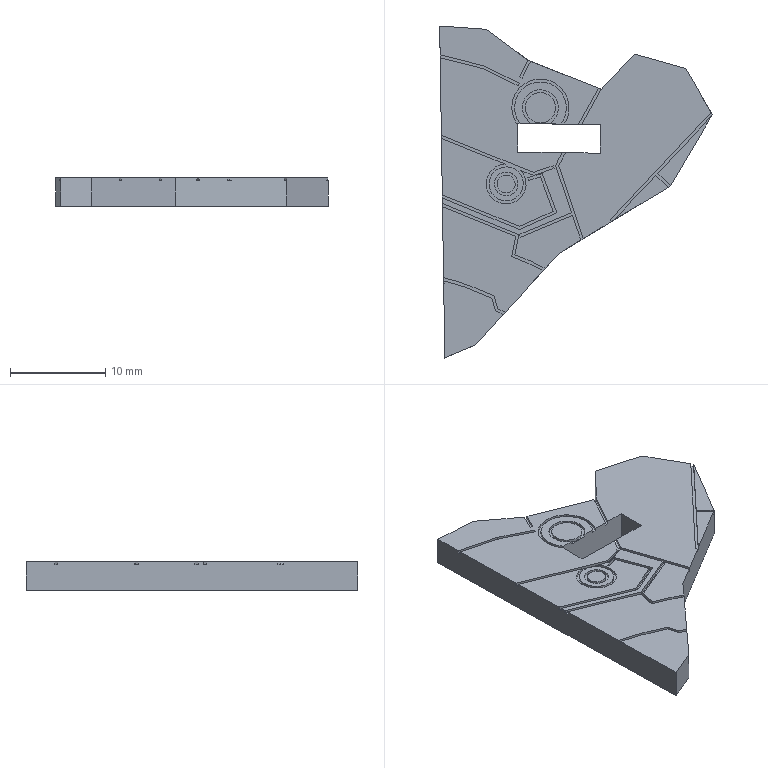Part | SolidWorks | features BaseBody 1 | 1 solid | 138 faces | box 28.565 x 34.776 x 3 mm | volume 1588 mm3 | plane 100 | spline 38